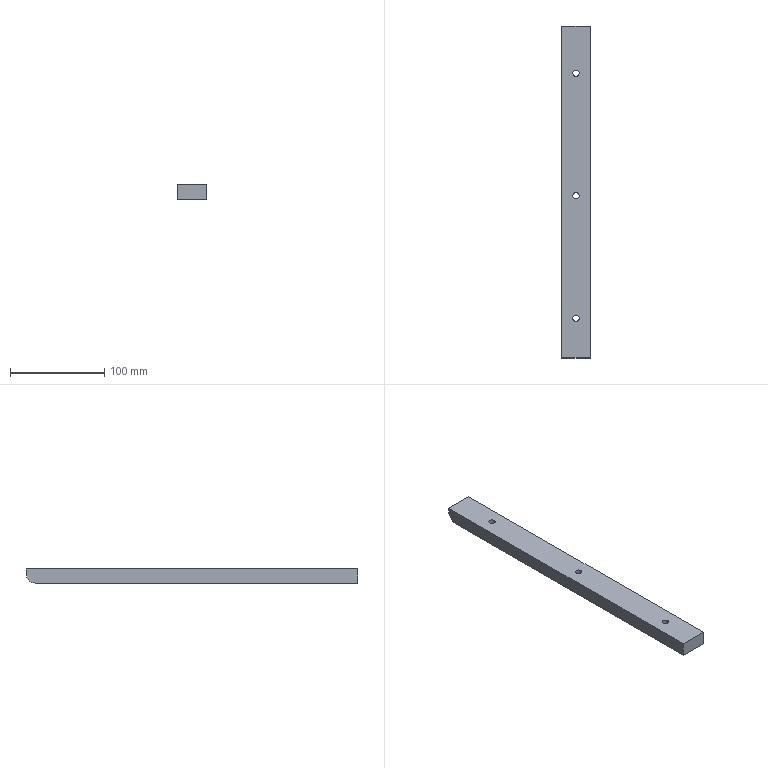Part | SolidWorks | features Extrusion 1, Fillet 1, HoleWzd 1 | 1 solid | 22 faces | box 30 x 352 x 15 mm | volume 154976 mm3 | cylinder 13 | plane 9 | commonest cylinder face diameters 6.6 x6 11 x6 20 x1
STEP:
#1=CARTESIAN_POINT('',(5.5,126.,6.8));
#2=VERTEX_POINT('',#1);
#3=CARTESIAN_POINT('',(-5.5,126.,6.8));
#4=VERTEX_POINT('',#3);
#5=CARTESIAN_POINT('',(0.,126.,6.8));
#6=DIRECTION('',(0.,0.,-1.));
#7=DIRECTION('',(-1.,0.,0.));
#8=AXIS2_PLACEMENT_3D('',#5,#6,#7);
#9=CIRCLE('',#8,5.5);
#10=EDGE_CURVE('',#2,#4,#9,.T.);
#11=ORIENTED_EDGE('',*,*,#10,.F.);
#12=CARTESIAN_POINT('',(5.5,126.,0.));
#13=VERTEX_POINT('',#12);
#14=CARTESIAN_POINT('',(5.5,126.,0.));
#15=DIRECTION('',(0.,0.,-1.));
#16=VECTOR('',#15,1000.);
#17=LINE('',#14,#16);
#18=EDGE_CURVE('',#2,#13,#17,.T.);
#19=ORIENTED_EDGE('',*,*,#18,.T.);
#20=CARTESIAN_POINT('',(-5.5,126.,0.));
#21=VERTEX_POINT('',#20);
#22=CARTESIAN_POINT('',(0.,126.,0.));
#23=DIRECTION('',(0.,0.,-1.));
#24=DIRECTION('',(-1.,0.,0.));
#25=AXIS2_PLACEMENT_3D('',#22,#23,#24);
#26=CIRCLE('',#25,5.5);
#27=EDGE_CURVE('',#13,#21,#26,.T.);
#28=ORIENTED_EDGE('',*,*,#27,.T.);
#29=CARTESIAN_POINT('',(-5.5,126.,0.));
#30=DIRECTION('',(0.,0.,-1.));
#31=VECTOR('',#30,1000.);
#32=LINE('',#29,#31);
#33=EDGE_CURVE('',#4,#21,#32,.T.);
#34=ORIENTED_EDGE('',*,*,#33,.F.);
#35=EDGE_LOOP('',(#11,#19,#28,#34));
#36=FACE_OUTER_BOUND('',#35,.T.);
#37=CARTESIAN_POINT('',(0.,126.,0.));
#38=DIRECTION('',(0.,0.,-1.));
#39=DIRECTION('',(-1.,0.,0.));
#40=AXIS2_PLACEMENT_3D('',#37,#38,#39);
#41=CYLINDRICAL_SURFACE('',#40,5.5);
#42=ADVANCED_FACE('',(#36),#41,.F.);
#43=CARTESIAN_POINT('',(3.3,126.,15.));
#44=VERTEX_POINT('',#43);
#45=CARTESIAN_POINT('',(-3.3,126.,15.));
#46=VERTEX_POINT('',#45);
#47=CARTESIAN_POINT('',(0.,126.,15.));
#48=DIRECTION('',(0.,0.,-1.));
#49=DIRECTION('',(-1.,0.,0.));
#50=AXIS2_PLACEMENT_3D('',#47,#48,#49);
#51=CIRCLE('',#50,3.3);
#52=EDGE_CURVE('',#44,#46,#51,.T.);
#53=ORIENTED_EDGE('',*,*,#52,.F.);
#54=CARTESIAN_POINT('',(3.3,126.,6.8));
#55=VERTEX_POINT('',#54);
#56=CARTESIAN_POINT('',(3.3,126.,0.));
#57=DIRECTION('',(0.,0.,-1.));
#58=VECTOR('',#57,1000.);
#59=LINE('',#56,#58);
#60=EDGE_CURVE('',#44,#55,#59,.T.);
#61=ORIENTED_EDGE('',*,*,#60,.T.);
#62=CARTESIAN_POINT('',(-3.3,126.,6.8));
#63=VERTEX_POINT('',#62);
#64=CARTESIAN_POINT('',(0.,126.,6.8));
#65=DIRECTION('',(0.,0.,-1.));
#66=DIRECTION('',(-1.,0.,0.));
#67=AXIS2_PLACEMENT_3D('',#64,#65,#66);
#68=CIRCLE('',#67,3.3);
#69=EDGE_CURVE('',#55,#63,#68,.T.);
#70=ORIENTED_EDGE('',*,*,#69,.T.);
#71=CARTESIAN_POINT('',(-3.3,126.,0.));
#72=DIRECTION('',(0.,0.,-1.));
#73=VECTOR('',#72,1000.);
#74=LINE('',#71,#73);
#75=EDGE_CURVE('',#46,#63,#74,.T.);
#76=ORIENTED_EDGE('',*,*,#75,.F.);
#77=EDGE_LOOP('',(#53,#61,#70,#76));
#78=FACE_OUTER_BOUND('',#77,.T.);
#79=CARTESIAN_POINT('',(0.,126.,0.));
#80=DIRECTION('',(0.,0.,-1.));
#81=DIRECTION('',(-1.,0.,0.));
#82=AXIS2_PLACEMENT_3D('',#79,#80,#81);
#83=CYLINDRICAL_SURFACE('',#82,3.3);
#84=ADVANCED_FACE('',(#78),#83,.F.);
#85=CARTESIAN_POINT('',(5.5,-4.,6.8));
#86=VERTEX_POINT('',#85);
#87=CARTESIAN_POINT('',(-5.5,-4.,6.8));
#88=VERTEX_POINT('',#87);
#89=CARTESIAN_POINT('',(0.,-4.,6.8));
#90=DIRECTION('',(0.,0.,-1.));
#91=DIRECTION('',(-1.,0.,0.));
#92=AXIS2_PLACEMENT_3D('',#89,#90,#91);
#93=CIRCLE('',#92,5.5);
#94=EDGE_CURVE('',#86,#88,#93,.T.);
#95=ORIENTED_EDGE('',*,*,#94,.F.);
#96=CARTESIAN_POINT('',(5.5,-4.,0.));
#97=VERTEX_POINT('',#96);
#98=CARTESIAN_POINT('',(5.5,-4.,0.));
#99=DIRECTION('',(0.,0.,-1.));
#100=VECTOR('',#99,1000.);
#101=LINE('',#98,#100);
#102=EDGE_CURVE('',#86,#97,#101,.T.);
#103=ORIENTED_EDGE('',*,*,#102,.T.);
#104=CARTESIAN_POINT('',(-5.5,-4.,0.));
#105=VERTEX_POINT('',#104);
#106=CARTESIAN_POINT('',(0.,-4.,0.));
#107=DIRECTION('',(0.,0.,-1.));
#108=DIRECTION('',(-1.,0.,0.));
#109=AXIS2_PLACEMENT_3D('',#106,#107,#108);
#110=CIRCLE('',#109,5.5);
#111=EDGE_CURVE('',#97,#105,#110,.T.);
#112=ORIENTED_EDGE('',*,*,#111,.T.);
#113=CARTESIAN_POINT('',(-5.5,-4.,0.));
#114=DIRECTION('',(0.,0.,-1.));
#115=VECTOR('',#114,1000.);
#116=LINE('',#113,#115);
#117=EDGE_CURVE('',#88,#105,#116,.T.);
#118=ORIENTED_EDGE('',*,*,#117,.F.);
#119=EDGE_LOOP('',(#95,#103,#112,#118));
#120=FACE_OUTER_BOUND('',#119,.T.);
#121=CARTESIAN_POINT('',(0.,-4.,0.));
#122=DIRECTION('',(0.,0.,-1.));
#123=DIRECTION('',(-1.,0.,0.));
#124=AXIS2_PLACEMENT_3D('',#121,#122,#123);
#125=CYLINDRICAL_SURFACE('',#124,5.5);
#126=ADVANCED_FACE('',(#120),#125,.F.);
#127=CARTESIAN_POINT('',(3.3,-4.,15.));
#128=VERTEX_POINT('',#127);
#129=CARTESIAN_POINT('',(-3.3,-4.,15.));
#130=VERTEX_POINT('',#129);
#131=CARTESIAN_POINT('',(0.,-4.,15.));
#132=DIRECTION('',(0.,0.,-1.));
#133=DIRECTION('',(-1.,0.,0.));
#134=AXIS2_PLACEMENT_3D('',#131,#132,#133);
#135=CIRCLE('',#134,3.3);
#136=EDGE_CURVE('',#128,#130,#135,.T.);
#137=ORIENTED_EDGE('',*,*,#136,.F.);
#138=CARTESIAN_POINT('',(3.3,-4.,6.8));
#139=VERTEX_POINT('',#138);
#140=CARTESIAN_POINT('',(3.3,-4.,0.));
#141=DIRECTION('',(0.,0.,-1.));
#142=VECTOR('',#141,1000.);
#143=LINE('',#140,#142);
#144=EDGE_CURVE('',#128,#139,#143,.T.);
#145=ORIENTED_EDGE('',*,*,#144,.T.);
#146=CARTESIAN_POINT('',(-3.3,-4.,6.8));
#147=VERTEX_POINT('',#146);
#148=CARTESIAN_POINT('',(0.,-4.,6.8));
#149=DIRECTION('',(0.,0.,-1.));
#150=DIRECTION('',(-1.,0.,0.));
#151=AXIS2_PLACEMENT_3D('',#148,#149,#150);
#152=CIRCLE('',#151,3.3);
#153=EDGE_CURVE('',#139,#147,#152,.T.);
#154=ORIENTED_EDGE('',*,*,#153,.T.);
#155=CARTESIAN_POINT('',(-3.3,-4.,0.));
#156=DIRECTION('',(0.,0.,-1.));
#157=VECTOR('',#156,1000.);
#158=LINE('',#155,#157);
#159=EDGE_CURVE('',#130,#147,#158,.T.);
#160=ORIENTED_EDGE('',*,*,#159,.F.);
#161=EDGE_LOOP('',(#137,#145,#154,#160));
#162=FACE_OUTER_BOUND('',#161,.T.);
#163=CARTESIAN_POINT('',(0.,-4.,0.));
#164=DIRECTION('',(0.,0.,-1.));
#165=DIRECTION('',(-1.,0.,0.));
#166=AXIS2_PLACEMENT_3D('',#163,#164,#165);
#167=CYLINDRICAL_SURFACE('',#166,3.3);
#168=ADVANCED_FACE('',(#162),#167,.F.);
#169=CARTESIAN_POINT('',(5.5,-134.,6.8));
#170=VERTEX_POINT('',#169);
#171=CARTESIAN_POINT('',(-5.5,-134.,6.8));
#172=VERTEX_POINT('',#171);
#173=CARTESIAN_POINT('',(0.,-134.,6.8));
#174=DIRECTION('',(0.,0.,-1.));
#175=DIRECTION('',(-1.,0.,0.));
#176=AXIS2_PLACEMENT_3D('',#173,#174,#175);
#177=CIRCLE('',#176,5.5);
#178=EDGE_CURVE('',#170,#172,#177,.T.);
#179=ORIENTED_EDGE('',*,*,#178,.F.);
#180=CARTESIAN_POINT('',(5.5,-134.,0.));
#181=VERTEX_POINT('',#180);
#182=CARTESIAN_POINT('',(5.5,-134.,0.));
#183=DIRECTION('',(0.,0.,-1.));
#184=VECTOR('',#183,1000.);
#185=LINE('',#182,#184);
#186=EDGE_CURVE('',#170,#181,#185,.T.);
#187=ORIENTED_EDGE('',*,*,#186,.T.);
#188=CARTESIAN_POINT('',(-5.5,-134.,0.));
#189=VERTEX_POINT('',#188);
#190=CARTESIAN_POINT('',(0.,-134.,0.));
#191=DIRECTION('',(0.,0.,-1.));
#192=DIRECTION('',(-1.,0.,0.));
#193=AXIS2_PLACEMENT_3D('',#190,#191,#192);
#194=CIRCLE('',#193,5.5);
#195=EDGE_CURVE('',#181,#189,#194,.T.);
#196=ORIENTED_EDGE('',*,*,#195,.T.);
#197=CARTESIAN_POINT('',(-5.5,-134.,0.));
#198=DIRECTION('',(0.,0.,-1.));
#199=VECTOR('',#198,1000.);
#200=LINE('',#197,#199);
#201=EDGE_CURVE('',#172,#189,#200,.T.);
#202=ORIENTED_EDGE('',*,*,#201,.F.);
#203=EDGE_LOOP('',(#179,#187,#196,#202));
#204=FACE_OUTER_BOUND('',#203,.T.);
#205=CARTESIAN_POINT('',(0.,-134.,0.));
#206=DIRECTION('',(0.,0.,-1.));
#207=DIRECTION('',(-1.,0.,0.));
#208=AXIS2_PLACEMENT_3D('',#205,#206,#207);
#209=CYLINDRICAL_SURFACE('',#208,5.5);
#210=ADVANCED_FACE('',(#204),#209,.F.);
#211=CARTESIAN_POINT('',(3.3,-134.,15.));
#212=VERTEX_POINT('',#211);
#213=CARTESIAN_POINT('',(-3.3,-134.,15.));
#214=VERTEX_POINT('',#213);
#215=CARTESIAN_POINT('',(0.,-134.,15.));
#216=DIRECTION('',(0.,0.,-1.));
#217=DIRECTION('',(-1.,0.,0.));
#218=AXIS2_PLACEMENT_3D('',#215,#216,#217);
#219=CIRCLE('',#218,3.3);
#220=EDGE_CURVE('',#212,#214,#219,.T.);
#221=ORIENTED_EDGE('',*,*,#220,.F.);
#222=CARTESIAN_POINT('',(3.3,-134.,6.8));
#223=VERTEX_POINT('',#222);
#224=CARTESIAN_POINT('',(3.3,-134.,0.));
#225=DIRECTION('',(0.,0.,-1.));
#226=VECTOR('',#225,1000.);
#227=LINE('',#224,#226);
#228=EDGE_CURVE('',#212,#223,#227,.T.);
#229=ORIENTED_EDGE('',*,*,#228,.T.);
#230=CARTESIAN_POINT('',(-3.3,-134.,6.8));
#231=VERTEX_POINT('',#230);
#232=CARTESIAN_POINT('',(0.,-134.,6.8));
#233=DIRECTION('',(0.,0.,-1.));
#234=DIRECTION('',(-1.,0.,0.));
#235=AXIS2_PLACEMENT_3D('',#232,#233,#234);
#236=CIRCLE('',#235,3.3);
#237=EDGE_CURVE('',#223,#231,#236,.T.);
#238=ORIENTED_EDGE('',*,*,#237,.T.);
#239=CARTESIAN_POINT('',(-3.3,-134.,0.));
#240=DIRECTION('',(0.,0.,-1.));
#241=VECTOR('',#240,1000.);
#242=LINE('',#239,#241);
#243=EDGE_CURVE('',#214,#231,#242,.T.);
#244=ORIENTED_EDGE('',*,*,#243,.F.);
#245=EDGE_LOOP('',(#221,#229,#238,#244));
#246=FACE_OUTER_BOUND('',#245,.T.);
#247=CARTESIAN_POINT('',(0.,-134.,0.));
#248=DIRECTION('',(0.,0.,-1.));
#249=DIRECTION('',(-1.,0.,0.));
#250=AXIS2_PLACEMENT_3D('',#247,#248,#249);
#251=CYLINDRICAL_SURFACE('',#250,3.3);
#252=ADVANCED_FACE('',(#246),#251,.F.);
#253=CARTESIAN_POINT('',(15.,-176.,0.));
#254=VERTEX_POINT('',#253);
#255=CARTESIAN_POINT('',(15.,166.,0.));
#256=VERTEX_POINT('',#255);
#257=CARTESIAN_POINT('',(15.,176.,0.));
#258=DIRECTION('',(0.,1.,0.));
#259=VECTOR('',#258,1000.);
#260=LINE('',#257,#259);
#261=EDGE_CURVE('',#254,#256,#260,.T.);
#262=ORIENTED_EDGE('',*,*,#261,.T.);
#263=CARTESIAN_POINT('',(15.,176.,10.));
#264=VERTEX_POINT('',#263);
#265=CARTESIAN_POINT('',(15.,166.,10.));
#266=DIRECTION('',(1.,0.,0.));
#267=DIRECTION('',(0.,-1.,0.));
#268=AXIS2_PLACEMENT_3D('',#265,#266,#267);
#269=CIRCLE('',#268,10.);
#270=EDGE_CURVE('',#256,#264,#269,.T.);
#271=ORIENTED_EDGE('',*,*,#270,.T.);
#272=CARTESIAN_POINT('',(15.,176.,15.));
#273=VERTEX_POINT('',#272);
#274=CARTESIAN_POINT('',(15.,176.,15.));
#275=DIRECTION('',(0.,0.,-1.));
#276=VECTOR('',#275,1000.);
#277=LINE('',#274,#276);
#278=EDGE_CURVE('',#273,#264,#277,.T.);
#279=ORIENTED_EDGE('',*,*,#278,.F.);
#280=CARTESIAN_POINT('',(15.,-176.,15.));
#281=VERTEX_POINT('',#280);
#282=CARTESIAN_POINT('',(15.,176.,15.));
#283=DIRECTION('',(0.,1.,0.));
#284=VECTOR('',#283,1000.);
#285=LINE('',#282,#284);
#286=EDGE_CURVE('',#281,#273,#285,.T.);
#287=ORIENTED_EDGE('',*,*,#286,.F.);
#288=CARTESIAN_POINT('',(15.,-176.,15.));
#289=DIRECTION('',(0.,0.,-1.));
#290=VECTOR('',#289,1000.);
#291=LINE('',#288,#290);
#292=EDGE_CURVE('',#281,#254,#291,.T.);
#293=ORIENTED_EDGE('',*,*,#292,.T.);
#294=EDGE_LOOP('',(#262,#271,#279,#287,#293));
#295=FACE_OUTER_BOUND('',#294,.T.);
#296=CARTESIAN_POINT('',(15.,176.,15.));
#297=DIRECTION('',(-1.,0.,0.));
#298=DIRECTION('',(0.,-1.,0.));
#299=AXIS2_PLACEMENT_3D('',#296,#297,#298);
#300=PLANE('',#299);
#301=ADVANCED_FACE('',(#295),#300,.F.);
#302=ORIENTED_EDGE('',*,*,#278,.T.);
#303=CARTESIAN_POINT('',(-15.,176.,10.));
#304=VERTEX_POINT('',#303);
#305=CARTESIAN_POINT('',(-15.,176.,10.));
#306=DIRECTION('',(-1.,0.,0.));
#307=VECTOR('',#306,1000.);
#308=LINE('',#305,#307);
#309=EDGE_CURVE('',#264,#304,#308,.T.);
#310=ORIENTED_EDGE('',*,*,#309,.T.);
#311=CARTESIAN_POINT('',(-15.,176.,15.));
#312=VERTEX_POINT('',#311);
#313=CARTESIAN_POINT('',(-15.,176.,15.));
#314=DIRECTION('',(0.,0.,-1.));
#315=VECTOR('',#314,1000.);
#316=LINE('',#313,#315);
#317=EDGE_CURVE('',#312,#304,#316,.T.);
#318=ORIENTED_EDGE('',*,*,#317,.F.);
#319=CARTESIAN_POINT('',(-15.,176.,15.));
#320=DIRECTION('',(-1.,0.,0.));
#321=VECTOR('',#320,1000.);
#322=LINE('',#319,#321);
#323=EDGE_CURVE('',#273,#312,#322,.T.);
#324=ORIENTED_EDGE('',*,*,#323,.F.);
#325=EDGE_LOOP('',(#302,#310,#318,#324));
#326=FACE_OUTER_BOUND('',#325,.T.);
#327=CARTESIAN_POINT('',(-15.,176.,15.));
#328=DIRECTION('',(0.,-1.,0.));
#329=DIRECTION('',(0.,0.,-1.));
#330=AXIS2_PLACEMENT_3D('',#327,#328,#329);
#331=PLANE('',#330);
#332=ADVANCED_FACE('',(#326),#331,.F.);
#333=ORIENTED_EDGE('',*,*,#317,.T.);
#334=CARTESIAN_POINT('',(-15.,166.,0.));
#335=VERTEX_POINT('',#334);
#336=CARTESIAN_POINT('',(-15.,166.,10.));
#337=DIRECTION('',(-1.,0.,0.));
#338=DIRECTION('',(0.,1.,0.));
#339=AXIS2_PLACEMENT_3D('',#336,#337,#338);
#340=CIRCLE('',#339,10.);
#341=EDGE_CURVE('',#304,#335,#340,.T.);
#342=ORIENTED_EDGE('',*,*,#341,.T.);
#343=CARTESIAN_POINT('',(-15.,-176.,0.));
#344=VERTEX_POINT('',#343);
#345=CARTESIAN_POINT('',(-15.,176.,0.));
#346=DIRECTION('',(0.,-1.,0.));
#347=VECTOR('',#346,1000.);
#348=LINE('',#345,#347);
#349=EDGE_CURVE('',#335,#344,#348,.T.);
#350=ORIENTED_EDGE('',*,*,#349,.T.);
#351=CARTESIAN_POINT('',(-15.,-176.,15.));
#352=VERTEX_POINT('',#351);
#353=CARTESIAN_POINT('',(-15.,-176.,15.));
#354=DIRECTION('',(0.,0.,-1.));
#355=VECTOR('',#354,1000.);
#356=LINE('',#353,#355);
#357=EDGE_CURVE('',#352,#344,#356,.T.);
#358=ORIENTED_EDGE('',*,*,#357,.F.);
#359=CARTESIAN_POINT('',(-15.,176.,15.));
#360=DIRECTION('',(0.,-1.,0.));
#361=VECTOR('',#360,1000.);
#362=LINE('',#359,#361);
#363=EDGE_CURVE('',#312,#352,#362,.T.);
#364=ORIENTED_EDGE('',*,*,#363,.F.);
#365=EDGE_LOOP('',(#333,#342,#350,#358,#364));
#366=FACE_OUTER_BOUND('',#365,.T.);
#367=CARTESIAN_POINT('',(-15.,176.,15.));
#368=DIRECTION('',(1.,0.,0.));
#369=DIRECTION('',(0.,1.,0.));
#370=AXIS2_PLACEMENT_3D('',#367,#368,#369);
#371=PLANE('',#370);
#372=ADVANCED_FACE('',(#366),#371,.F.);
#373=CARTESIAN_POINT('',(-15.,-176.,0.));
#374=DIRECTION('',(1.,0.,0.));
#375=VECTOR('',#374,1000.);
#376=LINE('',#373,#375);
#377=EDGE_CURVE('',#344,#254,#376,.T.);
#378=ORIENTED_EDGE('',*,*,#377,.T.);
#379=ORIENTED_EDGE('',*,*,#292,.F.);
#380=CARTESIAN_POINT('',(-15.,-176.,15.));
#381=DIRECTION('',(1.,0.,0.));
#382=VECTOR('',#381,1000.);
#383=LINE('',#380,#382);
#384=EDGE_CURVE('',#352,#281,#383,.T.);
#385=ORIENTED_EDGE('',*,*,#384,.F.);
#386=ORIENTED_EDGE('',*,*,#357,.T.);
#387=EDGE_LOOP('',(#378,#379,#385,#386));
#388=FACE_OUTER_BOUND('',#387,.T.);
#389=CARTESIAN_POINT('',(-15.,-176.,15.));
#390=DIRECTION('',(0.,1.,0.));
#391=DIRECTION('',(0.,0.,1.));
#392=AXIS2_PLACEMENT_3D('',#389,#390,#391);
#393=PLANE('',#392);
#394=ADVANCED_FACE('',(#388),#393,.F.);
#395=CARTESIAN_POINT('',(0.,126.,15.));
#396=DIRECTION('',(0.,0.,-1.));
#397=DIRECTION('',(-1.,0.,0.));
#398=AXIS2_PLACEMENT_3D('',#395,#396,#397);
#399=CIRCLE('',#398,3.3);
#400=EDGE_CURVE('',#46,#44,#399,.T.);
#401=ORIENTED_EDGE('',*,*,#400,.T.);
#402=ORIENTED_EDGE('',*,*,#52,.T.);
#403=EDGE_LOOP('',(#401,#402));
#404=FACE_BOUND('',#403,.T.);
#405=CARTESIAN_POINT('',(0.,-4.,15.));
#406=DIRECTION('',(0.,0.,-1.));
#407=DIRECTION('',(-1.,0.,0.));
#408=AXIS2_PLACEMENT_3D('',#405,#406,#407);
#409=CIRCLE('',#408,3.3);
#410=EDGE_CURVE('',#130,#128,#409,.T.);
#411=ORIENTED_EDGE('',*,*,#410,.T.);
#412=ORIENTED_EDGE('',*,*,#136,.T.);
#413=EDGE_LOOP('',(#411,#412));
#414=FACE_BOUND('',#413,.T.);
#415=CARTESIAN_POINT('',(0.,-134.,15.));
#416=DIRECTION('',(0.,0.,-1.));
#417=DIRECTION('',(-1.,0.,0.));
#418=AXIS2_PLACEMENT_3D('',#415,#416,#417);
#419=CIRCLE('',#418,3.3);
#420=EDGE_CURVE('',#214,#212,#419,.T.);
#421=ORIENTED_EDGE('',*,*,#420,.T.);
#422=ORIENTED_EDGE('',*,*,#220,.T.);
#423=EDGE_LOOP('',(#421,#422));
#424=FACE_BOUND('',#423,.T.);
#425=ORIENTED_EDGE('',*,*,#286,.T.);
#426=ORIENTED_EDGE('',*,*,#323,.T.);
#427=ORIENTED_EDGE('',*,*,#363,.T.);
#428=ORIENTED_EDGE('',*,*,#384,.T.);
#429=EDGE_LOOP('',(#425,#426,#427,#428));
#430=FACE_OUTER_BOUND('',#429,.T.);
#431=CARTESIAN_POINT('',(0.,0.,15.));
#432=DIRECTION('',(0.,0.,1.));
#433=DIRECTION('',(1.,0.,0.));
#434=AXIS2_PLACEMENT_3D('',#431,#432,#433);
#435=PLANE('',#434);
#436=ADVANCED_FACE('',(#404,#414,#424,#430),#435,.T.);
#437=CARTESIAN_POINT('',(0.,126.,0.));
#438=DIRECTION('',(0.,0.,-1.));
#439=DIRECTION('',(-1.,0.,0.));
#440=AXIS2_PLACEMENT_3D('',#437,#438,#439);
#441=CIRCLE('',#440,5.5);
#442=EDGE_CURVE('',#21,#13,#441,.T.);
#443=ORIENTED_EDGE('',*,*,#442,.F.);
#444=ORIENTED_EDGE('',*,*,#27,.F.);
#445=EDGE_LOOP('',(#443,#444));
#446=FACE_BOUND('',#445,.T.);
#447=CARTESIAN_POINT('',(0.,-4.,0.));
#448=DIRECTION('',(0.,0.,-1.));
#449=DIRECTION('',(-1.,0.,0.));
#450=AXIS2_PLACEMENT_3D('',#447,#448,#449);
#451=CIRCLE('',#450,5.5);
#452=EDGE_CURVE('',#105,#97,#451,.T.);
#453=ORIENTED_EDGE('',*,*,#452,.F.);
#454=ORIENTED_EDGE('',*,*,#111,.F.);
#455=EDGE_LOOP('',(#453,#454));
#456=FACE_BOUND('',#455,.T.);
#457=CARTESIAN_POINT('',(0.,-134.,0.));
#458=DIRECTION('',(0.,0.,-1.));
#459=DIRECTION('',(-1.,0.,0.));
#460=AXIS2_PLACEMENT_3D('',#457,#458,#459);
#461=CIRCLE('',#460,5.5);
#462=EDGE_CURVE('',#189,#181,#461,.T.);
#463=ORIENTED_EDGE('',*,*,#462,.F.);
#464=ORIENTED_EDGE('',*,*,#195,.F.);
#465=EDGE_LOOP('',(#463,#464));
#466=FACE_BOUND('',#465,.T.);
#467=ORIENTED_EDGE('',*,*,#349,.F.);
#468=CARTESIAN_POINT('',(0.,166.,0.));
#469=DIRECTION('',(1.,0.,0.));
#470=VECTOR('',#469,1000.);
#471=LINE('',#468,#470);
#472=EDGE_CURVE('',#335,#256,#471,.T.);
#473=ORIENTED_EDGE('',*,*,#472,.T.);
#474=ORIENTED_EDGE('',*,*,#261,.F.);
#475=ORIENTED_EDGE('',*,*,#377,.F.);
#476=EDGE_LOOP('',(#467,#473,#474,#475));
#477=FACE_OUTER_BOUND('',#476,.T.);
#478=CARTESIAN_POINT('',(0.,0.,0.));
#479=DIRECTION('',(0.,0.,1.));
#480=DIRECTION('',(1.,0.,0.));
#481=AXIS2_PLACEMENT_3D('',#478,#479,#480);
#482=PLANE('',#481);
#483=ADVANCED_FACE('',(#446,#456,#466,#477),#482,.F.);
#484=ORIENTED_EDGE('',*,*,#228,.F.);
#485=ORIENTED_EDGE('',*,*,#420,.F.);
#486=ORIENTED_EDGE('',*,*,#243,.T.);
#487=CARTESIAN_POINT('',(0.,-134.,6.8));
#488=DIRECTION('',(0.,0.,-1.));
#489=DIRECTION('',(-1.,0.,0.));
#490=AXIS2_PLACEMENT_3D('',#487,#488,#489);
#491=CIRCLE('',#490,3.3);
#492=EDGE_CURVE('',#231,#223,#491,.T.);
#493=ORIENTED_EDGE('',*,*,#492,.T.);
#494=EDGE_LOOP('',(#484,#485,#486,#493));
#495=FACE_OUTER_BOUND('',#494,.T.);
#496=CARTESIAN_POINT('',(0.,-134.,0.));
#497=DIRECTION('',(0.,0.,-1.));
#498=DIRECTION('',(-1.,0.,0.));
#499=AXIS2_PLACEMENT_3D('',#496,#497,#498);
#500=CYLINDRICAL_SURFACE('',#499,3.3);
#501=ADVANCED_FACE('',(#495),#500,.F.);
#502=ORIENTED_EDGE('',*,*,#492,.F.);
#503=ORIENTED_EDGE('',*,*,#237,.F.);
#504=EDGE_LOOP('',(#502,#503));
#505=FACE_BOUND('',#504,.T.);
#506=CARTESIAN_POINT('',(0.,-134.,6.8));
#507=DIRECTION('',(0.,0.,-1.));
#508=DIRECTION('',(-1.,0.,0.));
#509=AXIS2_PLACEMENT_3D('',#506,#507,#508);
#510=CIRCLE('',#509,5.5);
#511=EDGE_CURVE('',#172,#170,#510,.T.);
#512=ORIENTED_EDGE('',*,*,#511,.T.);
#513=ORIENTED_EDGE('',*,*,#178,.T.);
#514=EDGE_LOOP('',(#512,#513));
#515=FACE_OUTER_BOUND('',#514,.T.);
#516=CARTESIAN_POINT('',(3.3,-134.,6.8));
#517=DIRECTION('',(0.,0.,1.));
#518=DIRECTION('',(1.,0.,0.));
#519=AXIS2_PLACEMENT_3D('',#516,#517,#518);
#520=PLANE('',#519);
#521=ADVANCED_FACE('',(#505,#515),#520,.F.);
#522=ORIENTED_EDGE('',*,*,#186,.F.);
#523=ORIENTED_EDGE('',*,*,#511,.F.);
#524=ORIENTED_EDGE('',*,*,#201,.T.);
#525=ORIENTED_EDGE('',*,*,#462,.T.);
#526=EDGE_LOOP('',(#522,#523,#524,#525));
#527=FACE_OUTER_BOUND('',#526,.T.);
#528=CARTESIAN_POINT('',(0.,-134.,0.));
#529=DIRECTION('',(0.,0.,-1.));
#530=DIRECTION('',(-1.,0.,0.));
#531=AXIS2_PLACEMENT_3D('',#528,#529,#530);
#532=CYLINDRICAL_SURFACE('',#531,5.5);
#533=ADVANCED_FACE('',(#527),#532,.F.);
#534=ORIENTED_EDGE('',*,*,#144,.F.);
#535=ORIENTED_EDGE('',*,*,#410,.F.);
#536=ORIENTED_EDGE('',*,*,#159,.T.);
#537=CARTESIAN_POINT('',(0.,-4.,6.8));
#538=DIRECTION('',(0.,0.,-1.));
#539=DIRECTION('',(-1.,0.,0.));
#540=AXIS2_PLACEMENT_3D('',#537,#538,#539);
#541=CIRCLE('',#540,3.3);
#542=EDGE_CURVE('',#147,#139,#541,.T.);
#543=ORIENTED_EDGE('',*,*,#542,.T.);
#544=EDGE_LOOP('',(#534,#535,#536,#543));
#545=FACE_OUTER_BOUND('',#544,.T.);
#546=CARTESIAN_POINT('',(0.,-4.,0.));
#547=DIRECTION('',(0.,0.,-1.));
#548=DIRECTION('',(-1.,0.,0.));
#549=AXIS2_PLACEMENT_3D('',#546,#547,#548);
#550=CYLINDRICAL_SURFACE('',#549,3.3);
#551=ADVANCED_FACE('',(#545),#550,.F.);
#552=ORIENTED_EDGE('',*,*,#542,.F.);
#553=ORIENTED_EDGE('',*,*,#153,.F.);
#554=EDGE_LOOP('',(#552,#553));
#555=FACE_BOUND('',#554,.T.);
#556=CARTESIAN_POINT('',(0.,-4.,6.8));
#557=DIRECTION('',(0.,0.,-1.));
#558=DIRECTION('',(-1.,0.,0.));
#559=AXIS2_PLACEMENT_3D('',#556,#557,#558);
#560=CIRCLE('',#559,5.5);
#561=EDGE_CURVE('',#88,#86,#560,.T.);
#562=ORIENTED_EDGE('',*,*,#561,.T.);
#563=ORIENTED_EDGE('',*,*,#94,.T.);
#564=EDGE_LOOP('',(#562,#563));
#565=FACE_OUTER_BOUND('',#564,.T.);
#566=CARTESIAN_POINT('',(3.3,-4.,6.8));
#567=DIRECTION('',(0.,0.,1.));
#568=DIRECTION('',(1.,0.,0.));
#569=AXIS2_PLACEMENT_3D('',#566,#567,#568);
#570=PLANE('',#569);
#571=ADVANCED_FACE('',(#555,#565),#570,.F.);
#572=ORIENTED_EDGE('',*,*,#102,.F.);
#573=ORIENTED_EDGE('',*,*,#561,.F.);
#574=ORIENTED_EDGE('',*,*,#117,.T.);
#575=ORIENTED_EDGE('',*,*,#452,.T.);
#576=EDGE_LOOP('',(#572,#573,#574,#575));
#577=FACE_OUTER_BOUND('',#576,.T.);
#578=CARTESIAN_POINT('',(0.,-4.,0.));
#579=DIRECTION('',(0.,0.,-1.));
#580=DIRECTION('',(-1.,0.,0.));
#581=AXIS2_PLACEMENT_3D('',#578,#579,#580);
#582=CYLINDRICAL_SURFACE('',#581,5.5);
#583=ADVANCED_FACE('',(#577),#582,.F.);
#584=ORIENTED_EDGE('',*,*,#60,.F.);
#585=ORIENTED_EDGE('',*,*,#400,.F.);
#586=ORIENTED_EDGE('',*,*,#75,.T.);
#587=CARTESIAN_POINT('',(0.,126.,6.8));
#588=DIRECTION('',(0.,0.,-1.));
#589=DIRECTION('',(-1.,0.,0.));
#590=AXIS2_PLACEMENT_3D('',#587,#588,#589);
#591=CIRCLE('',#590,3.3);
#592=EDGE_CURVE('',#63,#55,#591,.T.);
#593=ORIENTED_EDGE('',*,*,#592,.T.);
#594=EDGE_LOOP('',(#584,#585,#586,#593));
#595=FACE_OUTER_BOUND('',#594,.T.);
#596=CARTESIAN_POINT('',(0.,126.,0.));
#597=DIRECTION('',(0.,0.,-1.));
#598=DIRECTION('',(-1.,0.,0.));
#599=AXIS2_PLACEMENT_3D('',#596,#597,#598);
#600=CYLINDRICAL_SURFACE('',#599,3.3);
#601=ADVANCED_FACE('',(#595),#600,.F.);
#602=ORIENTED_EDGE('',*,*,#592,.F.);
#603=ORIENTED_EDGE('',*,*,#69,.F.);
#604=EDGE_LOOP('',(#602,#603));
#605=FACE_BOUND('',#604,.T.);
#606=CARTESIAN_POINT('',(0.,126.,6.8));
#607=DIRECTION('',(0.,0.,-1.));
#608=DIRECTION('',(-1.,0.,0.));
#609=AXIS2_PLACEMENT_3D('',#606,#607,#608);
#610=CIRCLE('',#609,5.5);
#611=EDGE_CURVE('',#4,#2,#610,.T.);
#612=ORIENTED_EDGE('',*,*,#611,.T.);
#613=ORIENTED_EDGE('',*,*,#10,.T.);
#614=EDGE_LOOP('',(#612,#613));
#615=FACE_OUTER_BOUND('',#614,.T.);
#616=CARTESIAN_POINT('',(3.3,126.,6.8));
#617=DIRECTION('',(0.,0.,1.));
#618=DIRECTION('',(1.,0.,0.));
#619=AXIS2_PLACEMENT_3D('',#616,#617,#618);
#620=PLANE('',#619);
#621=ADVANCED_FACE('',(#605,#615),#620,.F.);
#622=ORIENTED_EDGE('',*,*,#18,.F.);
#623=ORIENTED_EDGE('',*,*,#611,.F.);
#624=ORIENTED_EDGE('',*,*,#33,.T.);
#625=ORIENTED_EDGE('',*,*,#442,.T.);
#626=EDGE_LOOP('',(#622,#623,#624,#625));
#627=FACE_OUTER_BOUND('',#626,.T.);
#628=CARTESIAN_POINT('',(0.,126.,0.));
#629=DIRECTION('',(0.,0.,-1.));
#630=DIRECTION('',(-1.,0.,0.));
#631=AXIS2_PLACEMENT_3D('',#628,#629,#630);
#632=CYLINDRICAL_SURFACE('',#631,5.5);
#633=ADVANCED_FACE('',(#627),#632,.F.);
#634=ORIENTED_EDGE('',*,*,#270,.F.);
#635=ORIENTED_EDGE('',*,*,#472,.F.);
#636=ORIENTED_EDGE('',*,*,#341,.F.);
#637=ORIENTED_EDGE('',*,*,#309,.F.);
#638=EDGE_LOOP('',(#634,#635,#636,#637));
#639=FACE_OUTER_BOUND('',#638,.T.);
#640=CARTESIAN_POINT('',(-15.,166.,10.));
#641=DIRECTION('',(-1.,0.,0.));
#642=DIRECTION('',(0.,0.,1.));
#643=AXIS2_PLACEMENT_3D('',#640,#641,#642);
#644=CYLINDRICAL_SURFACE('',#643,10.);
#645=ADVANCED_FACE('',(#639),#644,.T.);
#646=CLOSED_SHELL('',(#42,#84,#126,#168,#210,#252,#301,#332,#372,#394,#436,#483,#501,#521,#533,#551,#571,#583,#601,#621,#633,#645));
#647=MANIFOLD_SOLID_BREP('',#646);
#648=CARTESIAN_POINT('',(0.,0.,0.));
#649=DIRECTION('',(0.,0.,1.));
#650=DIRECTION('',(1.,0.,0.));
#651=AXIS2_PLACEMENT_3D('',#648,#649,#650);
#652=(LENGTH_UNIT()NAMED_UNIT(*)SI_UNIT(.MILLI.,.METRE.));
#653=UNCERTAINTY_MEASURE_WITH_UNIT(LENGTH_MEASURE(0.00001),#652,'','');
#654=(NAMED_UNIT(*)PLANE_ANGLE_UNIT()SI_UNIT($,.RADIAN.));
#655=(NAMED_UNIT(*)SI_UNIT($,.STERADIAN.)SOLID_ANGLE_UNIT());
#656=(GEOMETRIC_REPRESENTATION_CONTEXT(3)GLOBAL_UNCERTAINTY_ASSIGNED_CONTEXT((#653))GLOBAL_UNIT_ASSIGNED_CONTEXT((#652,#654,#655))REPRESENTATION_CONTEXT('',''));
#657=ADVANCED_BREP_SHAPE_REPRESENTATION('',(#647,#651),#656);